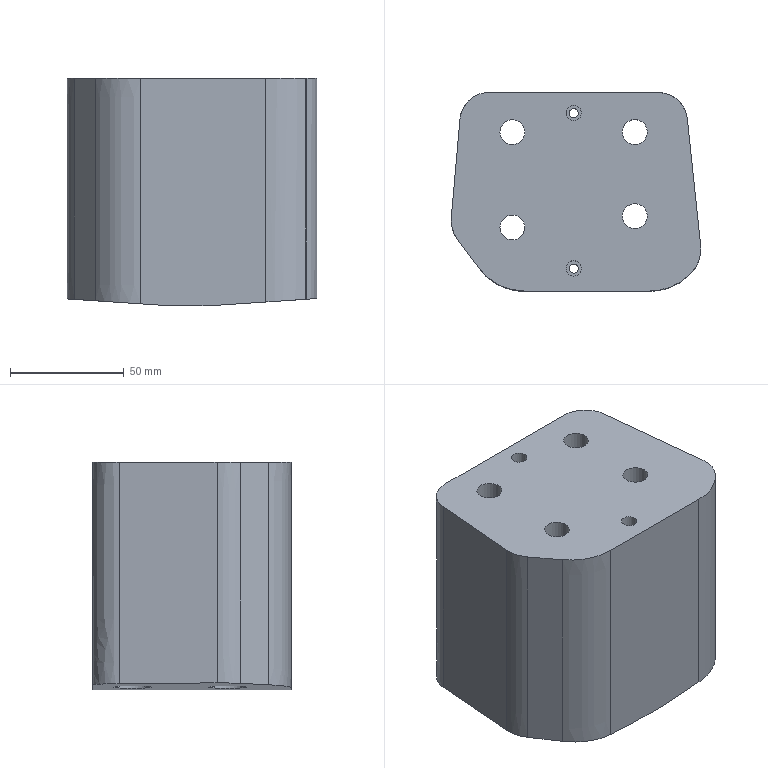Part | STEP file | lll_id3614_x_t | 1 solid | 42 faces | box 109.865 x 87.36 x 100 mm | volume 784858 mm3 | cylinder 18 | plane 18 | other 4 | cone 2 | commonest cylinder face diameters 11 x6 17 x4 4.1 x2 6.8 x2 8.506 x2 30 x1
STEP:
#1=CARTESIAN_POINT('',(3585.326,-140.05,29.5));
#2=VERTEX_POINT('',#1);
#3=CARTESIAN_POINT('',(3587.376,-140.05,29.5));
#4=DIRECTION('',(0.,0.,1.));
#5=DIRECTION('',(-1.,0.,0.));
#6=AXIS2_PLACEMENT_3D('',#3,#4,#5);
#7=CIRCLE('',#6,2.05);
#8=EDGE_CURVE('',#2,#2,#7,.T.);
#9=ORIENTED_EDGE('',*,*,#8,.T.);
#10=EDGE_LOOP('',(#9));
#11=FACE_BOUND('',#10,.T.);
#12=CARTESIAN_POINT('',(3587.376,-142.1,-7.5));
#13=VERTEX_POINT('',#12);
#14=CARTESIAN_POINT('',(3587.376,-140.05,-7.5));
#15=DIRECTION('',(0.,-0.000000008,-1.));
#16=DIRECTION('',(0.,-1.,0.000000008));
#17=AXIS2_PLACEMENT_3D('',#14,#15,#16);
#18=CIRCLE('',#17,2.05);
#19=EDGE_CURVE('',#13,#13,#18,.T.);
#20=ORIENTED_EDGE('',*,*,#19,.T.);
#21=EDGE_LOOP('',(#20));
#22=FACE_BOUND('',#21,.T.);
#23=CARTESIAN_POINT('',(3587.376,-140.05,42.5));
#24=DIRECTION('',(0.,0.,-1.));
#25=DIRECTION('',(0.,1.,0.));
#26=AXIS2_PLACEMENT_3D('',#23,#24,#25);
#27=CYLINDRICAL_SURFACE('',#26,2.05);
#28=ADVANCED_FACE('',(#11,#22),#27,.F.);
#29=CARTESIAN_POINT('',(3585.33,-71.615,29.5));
#30=VERTEX_POINT('',#29);
#31=CARTESIAN_POINT('',(3587.38,-71.615,29.5));
#32=DIRECTION('',(0.,0.,1.));
#33=DIRECTION('',(-1.,0.,0.));
#34=AXIS2_PLACEMENT_3D('',#31,#32,#33);
#35=CIRCLE('',#34,2.05);
#36=EDGE_CURVE('',#30,#30,#35,.T.);
#37=ORIENTED_EDGE('',*,*,#36,.T.);
#38=EDGE_LOOP('',(#37));
#39=FACE_BOUND('',#38,.T.);
#40=CARTESIAN_POINT('',(3587.38,-73.665,-7.5));
#41=VERTEX_POINT('',#40);
#42=CARTESIAN_POINT('',(3587.38,-71.615,-7.5));
#43=DIRECTION('',(0.,-0.000000008,-1.));
#44=DIRECTION('',(0.,-1.,0.000000008));
#45=AXIS2_PLACEMENT_3D('',#42,#43,#44);
#46=CIRCLE('',#45,2.05);
#47=EDGE_CURVE('',#41,#41,#46,.T.);
#48=ORIENTED_EDGE('',*,*,#47,.T.);
#49=EDGE_LOOP('',(#48));
#50=FACE_BOUND('',#49,.T.);
#51=CARTESIAN_POINT('',(3587.38,-71.615,42.5));
#52=DIRECTION('',(0.,0.,-1.));
#53=DIRECTION('',(-0.0006834,-1.,0.));
#54=AXIS2_PLACEMENT_3D('',#51,#52,#53);
#55=CYLINDRICAL_SURFACE('',#54,2.05);
#56=ADVANCED_FACE('',(#39,#50),#55,.F.);
#57=ORIENTED_EDGE('',*,*,#19,.F.);
#58=EDGE_LOOP('',(#57));
#59=FACE_BOUND('',#58,.T.);
#60=ORIENTED_EDGE('',*,*,#47,.F.);
#61=EDGE_LOOP('',(#60));
#62=FACE_BOUND('',#61,.T.);
#63=CARTESIAN_POINT('',(3587.38,-92.115,-7.5));
#64=VERTEX_POINT('',#63);
#65=CARTESIAN_POINT('',(3587.38,-86.615,-7.5));
#66=DIRECTION('',(0.,-0.000000008,-1.));
#67=DIRECTION('',(0.,-1.,0.000000008));
#68=AXIS2_PLACEMENT_3D('',#65,#66,#67);
#69=CIRCLE('',#68,5.5);
#70=EDGE_CURVE('',#64,#64,#69,.T.);
#71=ORIENTED_EDGE('',*,*,#70,.F.);
#72=EDGE_LOOP('',(#71));
#73=FACE_BOUND('',#72,.T.);
#74=CARTESIAN_POINT('',(3587.38,-130.115,-7.5));
#75=VERTEX_POINT('',#74);
#76=CARTESIAN_POINT('',(3587.38,-124.615,-7.5));
#77=DIRECTION('',(0.,-0.000000008,-1.));
#78=DIRECTION('',(0.,-1.,0.000000008));
#79=AXIS2_PLACEMENT_3D('',#76,#77,#78);
#80=CIRCLE('',#79,5.5);
#81=EDGE_CURVE('',#75,#75,#80,.T.);
#82=ORIENTED_EDGE('',*,*,#81,.F.);
#83=EDGE_LOOP('',(#82));
#84=FACE_BOUND('',#83,.T.);
#85=CARTESIAN_POINT('',(3597.232,-62.657,-7.5));
#86=VERTEX_POINT('',#85);
#87=CARTESIAN_POINT('',(3597.232,-150.017,-7.5));
#88=VERTEX_POINT('',#87);
#89=CARTESIAN_POINT('',(3597.232,-151.585,-7.5));
#90=DIRECTION('',(0.,-1.,0.));
#91=VECTOR('',#90,1.);
#92=LINE('',#89,#91);
#93=EDGE_CURVE('',#86,#88,#92,.T.);
#94=ORIENTED_EDGE('',*,*,#93,.T.);
#95=CARTESIAN_POINT('',(3577.232,-150.017,-7.5));
#96=VERTEX_POINT('',#95);
#97=CARTESIAN_POINT('',(3581.149,-150.017,-7.5));
#98=DIRECTION('',(-1.,0.,0.));
#99=VECTOR('',#98,1.);
#100=LINE('',#97,#99);
#101=EDGE_CURVE('',#88,#96,#100,.T.);
#102=ORIENTED_EDGE('',*,*,#101,.T.);
#103=CARTESIAN_POINT('',(3577.232,-62.657,-7.5));
#104=VERTEX_POINT('',#103);
#105=CARTESIAN_POINT('',(3577.232,-151.585,-7.5));
#106=DIRECTION('',(0.,-1.,0.));
#107=VECTOR('',#106,1.);
#108=LINE('',#105,#107);
#109=EDGE_CURVE('',#104,#96,#108,.T.);
#110=ORIENTED_EDGE('',*,*,#109,.F.);
#111=CARTESIAN_POINT('',(3587.337,-62.657,-7.5));
#112=DIRECTION('',(1.,0.,0.));
#113=VECTOR('',#112,1.);
#114=LINE('',#111,#113);
#115=EDGE_CURVE('',#104,#86,#114,.T.);
#116=ORIENTED_EDGE('',*,*,#115,.T.);
#117=EDGE_LOOP('',(#94,#102,#110,#116));
#118=FACE_BOUND('',#117,.T.);
#119=CARTESIAN_POINT('',(3633.202,65.944,-7.5));
#120=DIRECTION('',(0.,-0.000000008,1.));
#121=DIRECTION('',(0.,1.,0.000000008));
#122=AXIS2_PLACEMENT_3D('',#119,#120,#121);
#123=PLANE('',#122);
#124=ADVANCED_FACE('',(#59,#62,#73,#84,#118),#123,.F.);
#125=CARTESIAN_POINT('',(3638.938,-142.263,92.5));
#126=VERTEX_POINT('',#125);
#127=CARTESIAN_POINT('',(3638.507,-142.694,92.5));
#128=VERTEX_POINT('',#127);
#129=CARTESIAN_POINT('',(3802.568,21.366,92.5));
#130=DIRECTION('',(-0.7071,-0.7071,0.));
#131=VECTOR('',#130,1.);
#132=LINE('',#129,#131);
#133=EDGE_CURVE('',#126,#128,#132,.T.);
#134=ORIENTED_EDGE('',*,*,#133,.T.);
#135=CARTESIAN_POINT('',(3638.507,-142.694,-4.721));
#136=VERTEX_POINT('',#135);
#137=CARTESIAN_POINT('',(3638.507,-142.694,0.00002209));
#138=DIRECTION('',(0.000000008,0.,-1.));
#139=VECTOR('',#138,1.);
#140=LINE('',#137,#139);
#141=EDGE_CURVE('',#128,#136,#140,.T.);
#142=ORIENTED_EDGE('',*,*,#141,.T.);
#143=CARTESIAN_POINT('',(3638.938,-142.263,-4.692));
#144=VERTEX_POINT('',#143);
#145=CARTESIAN_POINT('',(3658.115,-123.087,-3.401));
#146=DIRECTION('',(0.7063,0.7063,0.04756));
#147=VECTOR('',#146,1.);
#148=LINE('',#145,#147);
#149=EDGE_CURVE('',#136,#144,#148,.T.);
#150=ORIENTED_EDGE('',*,*,#149,.T.);
#151=CARTESIAN_POINT('',(3638.938,-142.263,0.00002209));
#152=DIRECTION('',(-0.000000008,0.,1.));
#153=VECTOR('',#152,1.);
#154=LINE('',#151,#153);
#155=EDGE_CURVE('',#144,#126,#154,.T.);
#156=ORIENTED_EDGE('',*,*,#155,.T.);
#157=EDGE_LOOP('',(#134,#142,#150,#156));
#158=FACE_OUTER_BOUND('',#157,.T.);
#159=CARTESIAN_POINT('',(3638.507,-142.694,0.00002209));
#160=DIRECTION('',(-0.7071,0.7071,-0.000000005));
#161=DIRECTION('',(0.7071,0.7071,-0.000000005));
#162=AXIS2_PLACEMENT_3D('',#159,#160,#161);
#163=PLANE('',#162);
#164=ADVANCED_FACE('',(#158),#163,.F.);
#165=CARTESIAN_POINT('',(3637.367,-74.119,92.5));
#166=VERTEX_POINT('',#165);
#167=CARTESIAN_POINT('',(3643.25,-130.089,92.5));
#168=VERTEX_POINT('',#167);
#169=CARTESIAN_POINT('',(3639.152,-91.104,92.5));
#170=DIRECTION('',(0.1045,-0.9945,0.));
#171=VECTOR('',#170,1.);
#172=LINE('',#169,#171);
#173=EDGE_CURVE('',#166,#168,#172,.T.);
#174=ORIENTED_EDGE('',*,*,#173,.T.);
#175=CARTESIAN_POINT('',(3643.25,-130.089,-4.401));
#176=VERTEX_POINT('',#175);
#177=CARTESIAN_POINT('',(3643.25,-130.089,0.00001834));
#178=DIRECTION('',(0.000000008,0.,-1.));
#179=VECTOR('',#178,1.);
#180=LINE('',#177,#179);
#181=EDGE_CURVE('',#168,#176,#180,.T.);
#182=ORIENTED_EDGE('',*,*,#181,.T.);
#183=CARTESIAN_POINT('',(3637.367,-74.119,-4.798));
#184=VERTEX_POINT('',#183);
#185=CARTESIAN_POINT('',(3639.156,-91.136,-4.677));
#186=DIRECTION('',(-0.1045,0.9945,-0.007038));
#187=VECTOR('',#186,1.);
#188=LINE('',#185,#187);
#189=EDGE_CURVE('',#176,#184,#188,.T.);
#190=ORIENTED_EDGE('',*,*,#189,.T.);
#191=CARTESIAN_POINT('',(3637.367,-74.119,0.00001829));
#192=DIRECTION('',(-0.000000008,0.,1.));
#193=VECTOR('',#192,1.);
#194=LINE('',#191,#193);
#195=EDGE_CURVE('',#184,#166,#194,.T.);
#196=ORIENTED_EDGE('',*,*,#195,.T.);
#197=EDGE_LOOP('',(#174,#182,#190,#196));
#198=FACE_OUTER_BOUND('',#197,.T.);
#199=CARTESIAN_POINT('',(3639.152,-91.104,0.00001831));
#200=DIRECTION('',(-0.9945,-0.1045,-0.000000008));
#201=DIRECTION('',(0.1045,-0.9945,0.000000001));
#202=AXIS2_PLACEMENT_3D('',#199,#200,#201);
#203=PLANE('',#202);
#204=ADVANCED_FACE('',(#198),#203,.F.);
#205=ORIENTED_EDGE('',*,*,#195,.F.);
#206=CARTESIAN_POINT('',(3624.637,-62.657,-5.655));
#207=VERTEX_POINT('',#206);
#208=CARTESIAN_POINT('',(3637.367,-74.119,-4.798));
#209=CARTESIAN_POINT('',(3637.037,-70.978,-4.82));
#210=CARTESIAN_POINT('',(3635.528,-68.038,-4.921));
#211=CARTESIAN_POINT('',(3630.875,-63.85,-5.235));
#212=CARTESIAN_POINT('',(3627.791,-62.657,-5.442));
#213=CARTESIAN_POINT('',(3624.637,-62.657,-5.655));
#214=B_SPLINE_CURVE_WITH_KNOTS('',3,(#208,#209,#210,#211,#212,#213),.UNSPECIFIED.,.F.,.F.,(4,2,4),(0.,0.5,1.),.UNSPECIFIED.);
#215=EDGE_CURVE('',#184,#207,#214,.T.);
#216=ORIENTED_EDGE('',*,*,#215,.T.);
#217=CARTESIAN_POINT('',(3624.637,-62.657,92.5));
#218=VERTEX_POINT('',#217);
#219=CARTESIAN_POINT('',(3624.637,-62.657,0.0000182));
#220=DIRECTION('',(-0.000000008,0.,1.));
#221=VECTOR('',#220,1.);
#222=LINE('',#219,#221);
#223=EDGE_CURVE('',#207,#218,#222,.T.);
#224=ORIENTED_EDGE('',*,*,#223,.T.);
#225=CARTESIAN_POINT('',(3624.637,-62.657,92.5));
#226=CARTESIAN_POINT('',(3627.791,-62.657,92.5));
#227=CARTESIAN_POINT('',(3630.87,-63.847,92.5));
#228=CARTESIAN_POINT('',(3635.525,-68.034,92.5));
#229=CARTESIAN_POINT('',(3637.037,-70.978,92.5));
#230=CARTESIAN_POINT('',(3637.367,-74.119,92.5));
#231=B_SPLINE_CURVE_WITH_KNOTS('',3,(#225,#226,#227,#228,#229,#230),.UNSPECIFIED.,.F.,.F.,(4,2,4),(0.,0.5,1.),.UNSPECIFIED.);
#232=EDGE_CURVE('',#218,#166,#231,.T.);
#233=ORIENTED_EDGE('',*,*,#232,.T.);
#234=EDGE_LOOP('',(#205,#216,#224,#233));
#235=FACE_OUTER_BOUND('',#234,.T.);
#236=CARTESIAN_POINT('',(3624.637,-62.657,0.0000182));
#237=CARTESIAN_POINT('',(3625.028,-62.657,0.0000182));
#238=CARTESIAN_POINT('',(3625.81,-62.691,0.00001821));
#239=CARTESIAN_POINT('',(3627.361,-62.904,0.00001822));
#240=CARTESIAN_POINT('',(3629.249,-63.441,0.00001823));
#241=CARTESIAN_POINT('',(3631.364,-64.478,0.00001825));
#242=CARTESIAN_POINT('',(3633.249,-65.892,0.00001826));
#243=CARTESIAN_POINT('',(3634.852,-67.618,0.00001828));
#244=CARTESIAN_POINT('',(3636.105,-69.613,0.00001828));
#245=CARTESIAN_POINT('',(3636.836,-71.435,0.00001829));
#246=CARTESIAN_POINT('',(3637.21,-72.956,0.00001829));
#247=CARTESIAN_POINT('',(3637.326,-73.73,0.00001829));
#248=CARTESIAN_POINT('',(3637.367,-74.119,0.00001829));
#249=B_SPLINE_CURVE_WITH_KNOTS('',3,(#236,#237,#238,#239,#240,#241,#242,#243,#244,#245,#246,#247,#248),.UNSPECIFIED.,.F.,.F.,(4,1,1,1,1,1,1,1,1,1,4),(0.,0.0625,0.125,0.25,0.375,0.5,0.625,0.75,0.875,0.9375,1.),.UNSPECIFIED.);
#250=DIRECTION('',(-0.000000008,0.,1.));
#251=VECTOR('',#250,1.);
#252=SURFACE_OF_LINEAR_EXTRUSION('',#249,#251);
#253=ADVANCED_FACE('',(#235),#252,.F.);
#254=CARTESIAN_POINT('',(3550.037,-62.657,-5.669));
#255=VERTEX_POINT('',#254);
#256=CARTESIAN_POINT('',(3586.789,-62.657,-8.143));
#257=DIRECTION('',(0.9977,0.,-0.06718));
#258=VECTOR('',#257,1.);
#259=LINE('',#256,#258);
#260=EDGE_CURVE('',#255,#104,#259,.T.);
#261=ORIENTED_EDGE('',*,*,#260,.F.);
#262=CARTESIAN_POINT('',(3550.037,-62.657,92.5));
#263=VERTEX_POINT('',#262);
#264=CARTESIAN_POINT('',(3550.037,-62.657,0.00001763));
#265=DIRECTION('',(-0.000000008,0.,1.));
#266=VECTOR('',#265,1.);
#267=LINE('',#264,#266);
#268=EDGE_CURVE('',#255,#263,#267,.T.);
#269=ORIENTED_EDGE('',*,*,#268,.T.);
#270=CARTESIAN_POINT('',(3587.337,-62.657,92.5));
#271=DIRECTION('',(1.,0.,0.));
#272=VECTOR('',#271,1.);
#273=LINE('',#270,#272);
#274=EDGE_CURVE('',#263,#218,#273,.T.);
#275=ORIENTED_EDGE('',*,*,#274,.T.);
#276=ORIENTED_EDGE('',*,*,#223,.F.);
#277=CARTESIAN_POINT('',(3587.884,-62.657,-8.129));
#278=DIRECTION('',(-0.9977,0.,-0.06718));
#279=VECTOR('',#278,1.);
#280=LINE('',#277,#279);
#281=EDGE_CURVE('',#207,#86,#280,.T.);
#282=ORIENTED_EDGE('',*,*,#281,.T.);
#283=ORIENTED_EDGE('',*,*,#115,.F.);
#284=EDGE_LOOP('',(#261,#269,#275,#276,#282,#283));
#285=FACE_OUTER_BOUND('',#284,.T.);
#286=CARTESIAN_POINT('',(3587.337,-62.657,0.00001792));
#287=DIRECTION('',(0.,-1.,0.));
#288=DIRECTION('',(1.,0.,0.000000008));
#289=AXIS2_PLACEMENT_3D('',#286,#287,#288);
#290=PLANE('',#289);
#291=ADVANCED_FACE('',(#285),#290,.F.);
#292=CARTESIAN_POINT('',(3614.279,-71.531,62.5));
#293=VERTEX_POINT('',#292);
#294=CARTESIAN_POINT('',(3614.279,-80.031,62.5));
#295=DIRECTION('',(0.,0.,1.));
#296=DIRECTION('',(0.,1.,0.));
#297=AXIS2_PLACEMENT_3D('',#294,#295,#296);
#298=CIRCLE('',#297,8.5);
#299=EDGE_CURVE('',#293,#293,#298,.T.);
#300=ORIENTED_EDGE('',*,*,#299,.T.);
#301=EDGE_LOOP('',(#300));
#302=FACE_BOUND('',#301,.T.);
#303=CARTESIAN_POINT('',(3622.779,-80.031,-5.78));
#304=VERTEX_POINT('',#303);
#305=CARTESIAN_POINT('',(3614.279,-80.031,-6.352));
#306=DIRECTION('',(-0.06718,0.,0.9977));
#307=DIRECTION('',(0.9977,0.,0.06718));
#308=AXIS2_PLACEMENT_3D('',#305,#306,#307);
#309=ELLIPSE('',#308,8.519,8.5);
#310=EDGE_CURVE('',#304,#304,#309,.T.);
#311=ORIENTED_EDGE('',*,*,#310,.F.);
#312=EDGE_LOOP('',(#311));
#313=FACE_BOUND('',#312,.T.);
#314=CARTESIAN_POINT('',(3614.279,-80.031,12.5));
#315=DIRECTION('',(0.,0.,1.));
#316=DIRECTION('',(0.,-1.,0.));
#317=AXIS2_PLACEMENT_3D('',#314,#315,#316);
#318=CYLINDRICAL_SURFACE('',#317,8.5);
#319=ADVANCED_FACE('',(#302,#313),#318,.F.);
#320=CARTESIAN_POINT('',(3614.279,-108.531,62.5));
#321=VERTEX_POINT('',#320);
#322=CARTESIAN_POINT('',(3614.279,-117.031,62.5));
#323=DIRECTION('',(0.,0.,1.));
#324=DIRECTION('',(0.,1.,0.));
#325=AXIS2_PLACEMENT_3D('',#322,#323,#324);
#326=CIRCLE('',#325,8.5);
#327=EDGE_CURVE('',#321,#321,#326,.T.);
#328=ORIENTED_EDGE('',*,*,#327,.T.);
#329=EDGE_LOOP('',(#328));
#330=FACE_BOUND('',#329,.T.);
#331=CARTESIAN_POINT('',(3622.779,-117.031,-5.78));
#332=VERTEX_POINT('',#331);
#333=CARTESIAN_POINT('',(3614.279,-117.031,-6.352));
#334=DIRECTION('',(-0.06718,0.,0.9977));
#335=DIRECTION('',(0.9977,0.,0.06718));
#336=AXIS2_PLACEMENT_3D('',#333,#334,#335);
#337=ELLIPSE('',#336,8.519,8.5);
#338=EDGE_CURVE('',#332,#332,#337,.T.);
#339=ORIENTED_EDGE('',*,*,#338,.F.);
#340=EDGE_LOOP('',(#339));
#341=FACE_BOUND('',#340,.T.);
#342=CARTESIAN_POINT('',(3614.279,-117.031,12.5));
#343=DIRECTION('',(0.,0.,1.));
#344=DIRECTION('',(0.,-1.,0.));
#345=AXIS2_PLACEMENT_3D('',#342,#343,#344);
#346=CYLINDRICAL_SURFACE('',#345,8.5);
#347=ADVANCED_FACE('',(#330,#341),#346,.F.);
#348=CARTESIAN_POINT('',(3554.876,-80.05,92.5));
#349=VERTEX_POINT('',#348);
#350=CARTESIAN_POINT('',(3560.376,-80.05,92.5));
#351=DIRECTION('',(0.,0.,1.));
#352=DIRECTION('',(-1.,0.,0.));
#353=AXIS2_PLACEMENT_3D('',#350,#351,#352);
#354=CIRCLE('',#353,5.5);
#355=EDGE_CURVE('',#349,#349,#354,.T.);
#356=ORIENTED_EDGE('',*,*,#355,.F.);
#357=EDGE_LOOP('',(#356));
#358=FACE_BOUND('',#357,.T.);
#359=CARTESIAN_POINT('',(3620.83,-150.017,92.5));
#360=VERTEX_POINT('',#359);
#361=CARTESIAN_POINT('',(3565.78,-150.017,92.5));
#362=VERTEX_POINT('',#361);
#363=CARTESIAN_POINT('',(3581.149,-150.017,92.5));
#364=DIRECTION('',(-1.,0.,0.));
#365=VECTOR('',#364,1.);
#366=LINE('',#363,#365);
#367=EDGE_CURVE('',#360,#362,#366,.T.);
#368=ORIENTED_EDGE('',*,*,#367,.F.);
#369=CARTESIAN_POINT('',(3620.83,-125.017,92.5));
#370=DIRECTION('',(0.,0.,1.));
#371=DIRECTION('',(1.,0.,0.));
#372=AXIS2_PLACEMENT_3D('',#369,#370,#371);
#373=CIRCLE('',#372,25.);
#374=EDGE_CURVE('',#360,#128,#373,.T.);
#375=ORIENTED_EDGE('',*,*,#374,.T.);
#376=ORIENTED_EDGE('',*,*,#133,.F.);
#377=CARTESIAN_POINT('',(3628.332,-131.657,92.5));
#378=DIRECTION('',(0.,0.,1.));
#379=DIRECTION('',(1.,0.,0.));
#380=AXIS2_PLACEMENT_3D('',#377,#378,#379);
#381=CIRCLE('',#380,15.);
#382=EDGE_CURVE('',#126,#168,#381,.T.);
#383=ORIENTED_EDGE('',*,*,#382,.T.);
#384=ORIENTED_EDGE('',*,*,#173,.F.);
#385=ORIENTED_EDGE('',*,*,#232,.F.);
#386=ORIENTED_EDGE('',*,*,#274,.F.);
#387=CARTESIAN_POINT('',(3537.286,-74.341,92.5));
#388=VERTEX_POINT('',#387);
#389=CARTESIAN_POINT('',(3537.286,-74.341,92.5));
#390=CARTESIAN_POINT('',(3537.564,-71.162,92.5));
#391=CARTESIAN_POINT('',(3539.052,-68.163,92.5));
#392=CARTESIAN_POINT('',(3543.717,-63.885,92.5));
#393=CARTESIAN_POINT('',(3546.842,-62.657,92.5));
#394=CARTESIAN_POINT('',(3550.037,-62.657,92.5));
#395=B_SPLINE_CURVE_WITH_KNOTS('',3,(#389,#390,#391,#392,#393,#394),.UNSPECIFIED.,.F.,.F.,(4,2,4),(0.,0.5,1.),.UNSPECIFIED.);
#396=EDGE_CURVE('',#388,#263,#395,.T.);
#397=ORIENTED_EDGE('',*,*,#396,.F.);
#398=CARTESIAN_POINT('',(3533.523,-117.349,92.5));
#399=VERTEX_POINT('',#398);
#400=CARTESIAN_POINT('',(3535.404,-95.845,92.5));
#401=DIRECTION('',(0.08716,0.9962,0.));
#402=VECTOR('',#401,1.);
#403=LINE('',#400,#402);
#404=EDGE_CURVE('',#399,#388,#403,.T.);
#405=ORIENTED_EDGE('',*,*,#404,.F.);
#406=CARTESIAN_POINT('',(3536.486,-127.684,92.5));
#407=VERTEX_POINT('',#406);
#408=CARTESIAN_POINT('',(3536.486,-127.684,92.5));
#409=CARTESIAN_POINT('',(3534.267,-124.738,92.5));
#410=CARTESIAN_POINT('',(3533.202,-121.023,92.5));
#411=CARTESIAN_POINT('',(3533.523,-117.349,92.5));
#412=B_SPLINE_CURVE_WITH_KNOTS('',3,(#408,#409,#410,#411),.UNSPECIFIED.,.F.,.F.,(4,4),(0.,1.),.UNSPECIFIED.);
#413=EDGE_CURVE('',#407,#399,#412,.T.);
#414=ORIENTED_EDGE('',*,*,#413,.F.);
#415=CARTESIAN_POINT('',(3545.814,-140.062,92.5));
#416=VERTEX_POINT('',#415);
#417=CARTESIAN_POINT('',(3541.15,-133.873,92.5));
#418=DIRECTION('',(-0.6018,0.7986,0.));
#419=VECTOR('',#418,1.);
#420=LINE('',#417,#419);
#421=EDGE_CURVE('',#416,#407,#420,.T.);
#422=ORIENTED_EDGE('',*,*,#421,.F.);
#423=CARTESIAN_POINT('',(3565.78,-150.017,92.5));
#424=CARTESIAN_POINT('',(3561.891,-150.017,92.5));
#425=CARTESIAN_POINT('',(3558.048,-149.099,92.5));
#426=CARTESIAN_POINT('',(3552.892,-146.525,92.5));
#427=CARTESIAN_POINT('',(3551.245,-145.458,92.5));
#428=CARTESIAN_POINT('',(3548.301,-143.006,92.5));
#429=CARTESIAN_POINT('',(3546.983,-141.614,92.5));
#430=CARTESIAN_POINT('',(3545.814,-140.062,92.5));
#431=B_SPLINE_CURVE_WITH_KNOTS('',3,(#423,#424,#425,#426,#427,#428,#429,#430),.UNSPECIFIED.,.F.,.F.,(4,2,2,4),(0.,0.5,0.75,1.),.UNSPECIFIED.);
#432=EDGE_CURVE('',#362,#416,#431,.T.);
#433=ORIENTED_EDGE('',*,*,#432,.F.);
#434=EDGE_LOOP('',(#368,#375,#376,#383,#384,#385,#386,#397,#405,#414,#422,#433));
#435=FACE_BOUND('',#434,.T.);
#436=CARTESIAN_POINT('',(3587.378,-75.015,92.5));
#437=VERTEX_POINT('',#436);
#438=CARTESIAN_POINT('',(3587.38,-71.615,92.5));
#439=DIRECTION('',(0.,0.,-1.));
#440=DIRECTION('',(-0.0006834,-1.,0.));
#441=AXIS2_PLACEMENT_3D('',#438,#439,#440);
#442=CIRCLE('',#441,3.4);
#443=EDGE_CURVE('',#437,#437,#442,.T.);
#444=ORIENTED_EDGE('',*,*,#443,.T.);
#445=EDGE_LOOP('',(#444));
#446=FACE_BOUND('',#445,.T.);
#447=CARTESIAN_POINT('',(3587.376,-136.65,92.5));
#448=VERTEX_POINT('',#447);
#449=CARTESIAN_POINT('',(3587.376,-140.05,92.5));
#450=DIRECTION('',(0.,0.,1.));
#451=DIRECTION('',(0.,1.,0.));
#452=AXIS2_PLACEMENT_3D('',#449,#450,#451);
#453=CIRCLE('',#452,3.4);
#454=EDGE_CURVE('',#448,#448,#453,.T.);
#455=ORIENTED_EDGE('',*,*,#454,.F.);
#456=EDGE_LOOP('',(#455));
#457=FACE_BOUND('',#456,.T.);
#458=CARTESIAN_POINT('',(3608.779,-80.031,92.5));
#459=VERTEX_POINT('',#458);
#460=CARTESIAN_POINT('',(3614.279,-80.031,92.5));
#461=DIRECTION('',(0.,0.,-1.));
#462=DIRECTION('',(-1.,0.,0.));
#463=AXIS2_PLACEMENT_3D('',#460,#461,#462);
#464=CIRCLE('',#463,5.5);
#465=EDGE_CURVE('',#459,#459,#464,.T.);
#466=ORIENTED_EDGE('',*,*,#465,.T.);
#467=EDGE_LOOP('',(#466));
#468=FACE_BOUND('',#467,.T.);
#469=CARTESIAN_POINT('',(3608.779,-117.031,92.5));
#470=VERTEX_POINT('',#469);
#471=CARTESIAN_POINT('',(3614.279,-117.031,92.5));
#472=DIRECTION('',(0.,0.,-1.));
#473=DIRECTION('',(-1.,0.,0.));
#474=AXIS2_PLACEMENT_3D('',#471,#472,#473);
#475=CIRCLE('',#474,5.5);
#476=EDGE_CURVE('',#470,#470,#475,.T.);
#477=ORIENTED_EDGE('',*,*,#476,.T.);
#478=EDGE_LOOP('',(#477));
#479=FACE_BOUND('',#478,.T.);
#480=CARTESIAN_POINT('',(3554.876,-122.05,92.5));
#481=VERTEX_POINT('',#480);
#482=CARTESIAN_POINT('',(3560.376,-122.05,92.5));
#483=DIRECTION('',(0.,0.,-1.));
#484=DIRECTION('',(-1.,0.,0.));
#485=AXIS2_PLACEMENT_3D('',#482,#483,#484);
#486=CIRCLE('',#485,5.5);
#487=EDGE_CURVE('',#481,#481,#486,.T.);
#488=ORIENTED_EDGE('',*,*,#487,.T.);
#489=EDGE_LOOP('',(#488));
#490=FACE_BOUND('',#489,.T.);
#491=CARTESIAN_POINT('',(3587.234,236.7,92.5));
#492=DIRECTION('',(0.,0.,1.));
#493=DIRECTION('',(0.,-1.,0.));
#494=AXIS2_PLACEMENT_3D('',#491,#492,#493);
#495=PLANE('',#494);
#496=ADVANCED_FACE('',(#358,#435,#446,#457,#468,#479,#490),#495,.T.);
#497=CARTESIAN_POINT('',(3620.83,-150.017,-5.911));
#498=VERTEX_POINT('',#497);
#499=CARTESIAN_POINT('',(3581.724,-150.017,-8.544));
#500=DIRECTION('',(-0.9977,0.,-0.06718));
#501=VECTOR('',#500,1.);
#502=LINE('',#499,#501);
#503=EDGE_CURVE('',#498,#88,#502,.T.);
#504=ORIENTED_EDGE('',*,*,#503,.F.);
#505=CARTESIAN_POINT('',(3620.83,-150.017,0.00001817));
#506=DIRECTION('',(-0.000000008,0.,1.));
#507=VECTOR('',#506,1.);
#508=LINE('',#505,#507);
#509=EDGE_CURVE('',#498,#360,#508,.T.);
#510=ORIENTED_EDGE('',*,*,#509,.T.);
#511=ORIENTED_EDGE('',*,*,#367,.T.);
#512=CARTESIAN_POINT('',(3565.78,-150.017,-6.729));
#513=VERTEX_POINT('',#512);
#514=CARTESIAN_POINT('',(3565.78,-150.017,0.00001775));
#515=DIRECTION('',(-0.000000008,0.,1.));
#516=VECTOR('',#515,1.);
#517=LINE('',#514,#516);
#518=EDGE_CURVE('',#513,#362,#517,.T.);
#519=ORIENTED_EDGE('',*,*,#518,.F.);
#520=CARTESIAN_POINT('',(3580.628,-150.017,-7.729));
#521=DIRECTION('',(-0.9977,0.,0.06718));
#522=VECTOR('',#521,1.);
#523=LINE('',#520,#522);
#524=EDGE_CURVE('',#96,#513,#523,.T.);
#525=ORIENTED_EDGE('',*,*,#524,.F.);
#526=ORIENTED_EDGE('',*,*,#101,.F.);
#527=EDGE_LOOP('',(#504,#510,#511,#519,#525,#526));
#528=FACE_OUTER_BOUND('',#527,.T.);
#529=CARTESIAN_POINT('',(3581.149,-150.017,0.00001787));
#530=DIRECTION('',(0.,1.,0.));
#531=DIRECTION('',(-1.,0.,-0.000000008));
#532=AXIS2_PLACEMENT_3D('',#529,#530,#531);
#533=PLANE('',#532);
#534=ADVANCED_FACE('',(#528),#533,.F.);
#535=CARTESIAN_POINT('',(3537.286,-74.341,-4.81));
#536=VERTEX_POINT('',#535);
#537=CARTESIAN_POINT('',(3550.037,-62.657,-5.669));
#538=CARTESIAN_POINT('',(3546.849,-62.657,-5.454));
#539=CARTESIAN_POINT('',(3543.735,-63.874,-5.245));
#540=CARTESIAN_POINT('',(3539.063,-68.147,-4.93));
#541=CARTESIAN_POINT('',(3537.565,-71.154,-4.829));
#542=CARTESIAN_POINT('',(3537.286,-74.341,-4.81));
#543=B_SPLINE_CURVE_WITH_KNOTS('',3,(#537,#538,#539,#540,#541,#542),.UNSPECIFIED.,.F.,.F.,(4,2,4),(0.,0.5,1.),.UNSPECIFIED.);
#544=EDGE_CURVE('',#255,#536,#543,.T.);
#545=ORIENTED_EDGE('',*,*,#544,.T.);
#546=CARTESIAN_POINT('',(3537.286,-74.341,0.00001754));
#547=DIRECTION('',(-0.000000008,0.,1.));
#548=VECTOR('',#547,1.);
#549=LINE('',#546,#548);
#550=EDGE_CURVE('',#536,#388,#549,.T.);
#551=ORIENTED_EDGE('',*,*,#550,.T.);
#552=ORIENTED_EDGE('',*,*,#396,.T.);
#553=ORIENTED_EDGE('',*,*,#268,.F.);
#554=EDGE_LOOP('',(#545,#551,#552,#553));
#555=FACE_OUTER_BOUND('',#554,.T.);
#556=CARTESIAN_POINT('',(3537.286,-74.341,0.00001754));
#557=CARTESIAN_POINT('',(3537.32,-73.947,0.00001754));
#558=CARTESIAN_POINT('',(3537.425,-73.162,0.00001754));
#559=CARTESIAN_POINT('',(3537.778,-71.617,0.00001754));
#560=CARTESIAN_POINT('',(3538.492,-69.763,0.00001755));
#561=CARTESIAN_POINT('',(3539.736,-67.729,0.00001755));
#562=CARTESIAN_POINT('',(3541.341,-65.967,0.00001757));
#563=CARTESIAN_POINT('',(3543.237,-64.521,0.00001758));
#564=CARTESIAN_POINT('',(3545.372,-63.46,0.0000176));
#565=CARTESIAN_POINT('',(3547.281,-62.91,0.00001761));
#566=CARTESIAN_POINT('',(3548.85,-62.692,0.00001762));
#567=CARTESIAN_POINT('',(3549.641,-62.657,0.00001763));
#568=CARTESIAN_POINT('',(3550.037,-62.657,0.00001763));
#569=B_SPLINE_CURVE_WITH_KNOTS('',3,(#556,#557,#558,#559,#560,#561,#562,#563,#564,#565,#566,#567,#568),.UNSPECIFIED.,.F.,.F.,(4,1,1,1,1,1,1,1,1,1,4),(0.,0.0625,0.125,0.25,0.375,0.5,0.625,0.75,0.875,0.9375,1.),.UNSPECIFIED.);
#570=DIRECTION('',(-0.000000008,0.,1.));
#571=VECTOR('',#570,1.);
#572=SURFACE_OF_LINEAR_EXTRUSION('',#569,#571);
#573=ADVANCED_FACE('',(#555),#572,.F.);
#574=CARTESIAN_POINT('',(3533.523,-117.349,-4.557));
#575=VERTEX_POINT('',#574);
#576=CARTESIAN_POINT('',(3535.402,-95.872,-4.683));
#577=DIRECTION('',(-0.08715,-0.9962,0.005868));
#578=VECTOR('',#577,1.);
#579=LINE('',#576,#578);
#580=EDGE_CURVE('',#536,#575,#579,.T.);
#581=ORIENTED_EDGE('',*,*,#580,.T.);
#582=CARTESIAN_POINT('',(3533.523,-117.349,0.00001751));
#583=DIRECTION('',(-0.000000008,0.,1.));
#584=VECTOR('',#583,1.);
#585=LINE('',#582,#584);
#586=EDGE_CURVE('',#575,#399,#585,.T.);
#587=ORIENTED_EDGE('',*,*,#586,.T.);
#588=ORIENTED_EDGE('',*,*,#404,.T.);
#589=ORIENTED_EDGE('',*,*,#550,.F.);
#590=EDGE_LOOP('',(#581,#587,#588,#589));
#591=FACE_OUTER_BOUND('',#590,.T.);
#592=CARTESIAN_POINT('',(3535.404,-95.845,0.00001752));
#593=DIRECTION('',(0.9962,-0.08716,0.000000008));
#594=DIRECTION('',(0.08716,0.9962,0.000000001));
#595=AXIS2_PLACEMENT_3D('',#592,#593,#594);
#596=PLANE('',#595);
#597=ADVANCED_FACE('',(#591),#596,.F.);
#598=CARTESIAN_POINT('',(3536.486,-127.684,-4.756));
#599=VERTEX_POINT('',#598);
#600=CARTESIAN_POINT('',(3533.523,-117.349,-4.557));
#601=CARTESIAN_POINT('',(3533.202,-121.024,-4.535));
#602=CARTESIAN_POINT('',(3534.268,-124.74,-4.607));
#603=CARTESIAN_POINT('',(3536.486,-127.684,-4.756));
#604=B_SPLINE_CURVE_WITH_KNOTS('',3,(#600,#601,#602,#603),.UNSPECIFIED.,.F.,.F.,(4,4),(0.,1.),.UNSPECIFIED.);
#605=EDGE_CURVE('',#575,#599,#604,.T.);
#606=ORIENTED_EDGE('',*,*,#605,.T.);
#607=CARTESIAN_POINT('',(3536.486,-127.684,0.00001753));
#608=DIRECTION('',(-0.000000008,0.,1.));
#609=VECTOR('',#608,1.);
#610=LINE('',#607,#609);
#611=EDGE_CURVE('',#599,#407,#610,.T.);
#612=ORIENTED_EDGE('',*,*,#611,.T.);
#613=ORIENTED_EDGE('',*,*,#413,.T.);
#614=ORIENTED_EDGE('',*,*,#586,.F.);
#615=EDGE_LOOP('',(#606,#612,#613,#614));
#616=FACE_OUTER_BOUND('',#615,.T.);
#617=CARTESIAN_POINT('',(3536.486,-127.684,0.00001753));
#618=CARTESIAN_POINT('',(3536.211,-127.318,0.00001753));
#619=CARTESIAN_POINT('',(3535.692,-126.561,0.00001752));
#620=CARTESIAN_POINT('',(3535.021,-125.36,0.00001752));
#621=CARTESIAN_POINT('',(3534.465,-124.101,0.00001751));
#622=CARTESIAN_POINT('',(3534.027,-122.797,0.00001751));
#623=CARTESIAN_POINT('',(3533.707,-121.458,0.00001751));
#624=CARTESIAN_POINT('',(3533.511,-120.096,0.00001751));
#625=CARTESIAN_POINT('',(3533.444,-118.722,0.00001751));
#626=CARTESIAN_POINT('',(3533.483,-117.806,0.00001751));
#627=CARTESIAN_POINT('',(3533.523,-117.349,0.00001751));
#628=B_SPLINE_CURVE_WITH_KNOTS('',3,(#617,#618,#619,#620,#621,#622,#623,#624,#625,#626,#627),.UNSPECIFIED.,.F.,.F.,(4,1,1,1,1,1,1,1,4),(0.,0.125,0.25,0.375,0.5,0.625,0.75,0.875,1.),.UNSPECIFIED.);
#629=DIRECTION('',(-0.000000008,0.,1.));
#630=VECTOR('',#629,1.);
#631=SURFACE_OF_LINEAR_EXTRUSION('',#628,#630);
#632=ADVANCED_FACE('',(#616),#631,.F.);
#633=CARTESIAN_POINT('',(3545.814,-140.062,-5.385));
#634=VERTEX_POINT('',#633);
#635=CARTESIAN_POINT('',(3541.027,-133.709,-5.062));
#636=DIRECTION('',(0.6013,-0.798,-0.04049));
#637=VECTOR('',#636,1.);
#638=LINE('',#635,#637);
#639=EDGE_CURVE('',#599,#634,#638,.T.);
#640=ORIENTED_EDGE('',*,*,#639,.T.);
#641=CARTESIAN_POINT('',(3545.814,-140.062,0.0000176));
#642=DIRECTION('',(-0.000000008,0.,1.));
#643=VECTOR('',#642,1.);
#644=LINE('',#641,#643);
#645=EDGE_CURVE('',#634,#416,#644,.T.);
#646=ORIENTED_EDGE('',*,*,#645,.T.);
#647=ORIENTED_EDGE('',*,*,#421,.T.);
#648=ORIENTED_EDGE('',*,*,#611,.F.);
#649=EDGE_LOOP('',(#640,#646,#647,#648));
#650=FACE_OUTER_BOUND('',#649,.T.);
#651=CARTESIAN_POINT('',(3541.15,-133.873,0.00001757));
#652=DIRECTION('',(0.7986,0.6018,0.000000006));
#653=DIRECTION('',(-0.6018,0.7986,-0.000000005));
#654=AXIS2_PLACEMENT_3D('',#651,#652,#653);
#655=PLANE('',#654);
#656=ADVANCED_FACE('',(#650),#655,.F.);
#657=CARTESIAN_POINT('',(3545.814,-140.062,-5.385));
#658=CARTESIAN_POINT('',(3548.156,-143.17,-5.542));
#659=CARTESIAN_POINT('',(3551.204,-145.688,-5.747));
#660=CARTESIAN_POINT('',(3556.362,-148.255,-6.095));
#661=CARTESIAN_POINT('',(3558.205,-148.928,-6.219));
#662=CARTESIAN_POINT('',(3561.934,-149.803,-6.47));
#663=CARTESIAN_POINT('',(3563.838,-150.017,-6.598));
#664=CARTESIAN_POINT('',(3565.78,-150.017,-6.729));
#665=B_SPLINE_CURVE_WITH_KNOTS('',3,(#657,#658,#659,#660,#661,#662,#663,#664),.UNSPECIFIED.,.F.,.F.,(4,2,2,4),(0.,0.5,0.75,1.),.UNSPECIFIED.);
#666=EDGE_CURVE('',#634,#513,#665,.T.);
#667=ORIENTED_EDGE('',*,*,#666,.T.);
#668=ORIENTED_EDGE('',*,*,#518,.T.);
#669=ORIENTED_EDGE('',*,*,#432,.T.);
#670=ORIENTED_EDGE('',*,*,#645,.F.);
#671=EDGE_LOOP('',(#667,#668,#669,#670));
#672=FACE_OUTER_BOUND('',#671,.T.);
#673=CARTESIAN_POINT('',(3565.78,-150.017,0.00001775));
#674=CARTESIAN_POINT('',(3565.298,-150.017,0.00001775));
#675=CARTESIAN_POINT('',(3564.334,-149.99,0.00001774));
#676=CARTESIAN_POINT('',(3562.413,-149.828,0.00001773));
#677=CARTESIAN_POINT('',(3560.034,-149.416,0.00001771));
#678=CARTESIAN_POINT('',(3557.723,-148.723,0.00001769));
#679=CARTESIAN_POINT('',(3555.931,-148.011,0.00001768));
#680=CARTESIAN_POINT('',(3554.619,-147.402,0.00001767));
#681=CARTESIAN_POINT('',(3553.343,-146.721,0.00001766));
#682=CARTESIAN_POINT('',(3551.696,-145.718,0.00001765));
#683=CARTESIAN_POINT('',(3549.751,-144.289,0.00001763));
#684=CARTESIAN_POINT('',(3547.991,-142.638,0.00001762));
#685=CARTESIAN_POINT('',(3546.705,-141.201,0.00001761));
#686=CARTESIAN_POINT('',(3546.104,-140.447,0.0000176));
#687=CARTESIAN_POINT('',(3545.814,-140.062,0.0000176));
#688=B_SPLINE_CURVE_WITH_KNOTS('',3,(#673,#674,#675,#676,#677,#678,#679,#680,#681,#682,#683,#684,#685,#686,#687),.UNSPECIFIED.,.F.,.F.,(4,1,1,1,1,1,1,1,1,1,1,1,4),(0.,0.0625,0.125,0.25,0.375,0.4375,0.5,0.5625,0.625,0.75,0.875,0.9375,1.),.UNSPECIFIED.);
#689=DIRECTION('',(-0.000000008,0.,1.));
#690=VECTOR('',#689,1.);
#691=SURFACE_OF_LINEAR_EXTRUSION('',#688,#690);
#692=ADVANCED_FACE('',(#672),#691,.F.);
#693=ORIENTED_EDGE('',*,*,#454,.T.);
#694=EDGE_LOOP('',(#693));
#695=FACE_BOUND('',#694,.T.);
#696=CARTESIAN_POINT('',(3587.376,-143.45,29.5));
#697=VERTEX_POINT('',#696);
#698=CARTESIAN_POINT('',(3587.376,-140.05,29.5));
#699=DIRECTION('',(0.,0.,1.));
#700=DIRECTION('',(0.,-1.,0.));
#701=AXIS2_PLACEMENT_3D('',#698,#699,#700);
#702=CIRCLE('',#701,3.4);
#703=EDGE_CURVE('',#697,#697,#702,.T.);
#704=ORIENTED_EDGE('',*,*,#703,.F.);
#705=EDGE_LOOP('',(#704));
#706=FACE_BOUND('',#705,.T.);
#707=CARTESIAN_POINT('',(3587.376,-140.05,42.5));
#708=DIRECTION('',(0.,0.,1.));
#709=DIRECTION('',(0.,-1.,0.));
#710=AXIS2_PLACEMENT_3D('',#707,#708,#709);
#711=CYLINDRICAL_SURFACE('',#710,3.4);
#712=ADVANCED_FACE('',(#695,#706),#711,.F.);
#713=CARTESIAN_POINT('',(3608.779,-80.031,62.5));
#714=VERTEX_POINT('',#713);
#715=CARTESIAN_POINT('',(3614.279,-80.031,62.5));
#716=DIRECTION('',(0.,0.,1.));
#717=DIRECTION('',(-1.,0.,0.));
#718=AXIS2_PLACEMENT_3D('',#715,#716,#717);
#719=CIRCLE('',#718,5.5);
#720=EDGE_CURVE('',#714,#714,#719,.T.);
#721=ORIENTED_EDGE('',*,*,#720,.F.);
#722=EDGE_LOOP('',(#721));
#723=FACE_BOUND('',#722,.T.);
#724=ORIENTED_EDGE('',*,*,#465,.F.);
#725=EDGE_LOOP('',(#724));
#726=FACE_BOUND('',#725,.T.);
#727=CARTESIAN_POINT('',(3614.279,-80.031,112.5));
#728=DIRECTION('',(0.,0.,-1.));
#729=DIRECTION('',(0.,1.,0.));
#730=AXIS2_PLACEMENT_3D('',#727,#728,#729);
#731=CYLINDRICAL_SURFACE('',#730,5.5);
#732=ADVANCED_FACE('',(#723,#726),#731,.F.);
#733=ORIENTED_EDGE('',*,*,#299,.F.);
#734=EDGE_LOOP('',(#733));
#735=FACE_BOUND('',#734,.T.);
#736=ORIENTED_EDGE('',*,*,#720,.T.);
#737=EDGE_LOOP('',(#736));
#738=FACE_BOUND('',#737,.T.);
#739=CARTESIAN_POINT('',(3614.279,-80.031,62.5));
#740=DIRECTION('',(0.,0.,1.));
#741=DIRECTION('',(0.,-1.,0.));
#742=AXIS2_PLACEMENT_3D('',#739,#740,#741);
#743=PLANE('',#742);
#744=ADVANCED_FACE('',(#735,#738),#743,.F.);
#745=ORIENTED_EDGE('',*,*,#443,.F.);
#746=EDGE_LOOP('',(#745));
#747=FACE_BOUND('',#746,.T.);
#748=CARTESIAN_POINT('',(3587.382,-68.215,29.5));
#749=VERTEX_POINT('',#748);
#750=CARTESIAN_POINT('',(3587.38,-71.615,29.5));
#751=DIRECTION('',(0.,0.,-1.));
#752=DIRECTION('',(0.0006834,1.,0.));
#753=AXIS2_PLACEMENT_3D('',#750,#751,#752);
#754=CIRCLE('',#753,3.4);
#755=EDGE_CURVE('',#749,#749,#754,.T.);
#756=ORIENTED_EDGE('',*,*,#755,.T.);
#757=EDGE_LOOP('',(#756));
#758=FACE_BOUND('',#757,.T.);
#759=CARTESIAN_POINT('',(3587.38,-71.615,42.5));
#760=DIRECTION('',(0.,0.,1.));
#761=DIRECTION('',(0.0006834,1.,0.));
#762=AXIS2_PLACEMENT_3D('',#759,#760,#761);
#763=CYLINDRICAL_SURFACE('',#762,3.4);
#764=ADVANCED_FACE('',(#747,#758),#763,.F.);
#765=CARTESIAN_POINT('',(3554.876,-80.05,62.5));
#766=VERTEX_POINT('',#765);
#767=CARTESIAN_POINT('',(3560.376,-80.05,62.5));
#768=DIRECTION('',(0.,0.,1.));
#769=DIRECTION('',(-1.,0.,0.));
#770=AXIS2_PLACEMENT_3D('',#767,#768,#769);
#771=CIRCLE('',#770,5.5);
#772=EDGE_CURVE('',#766,#766,#771,.T.);
#773=ORIENTED_EDGE('',*,*,#772,.F.);
#774=EDGE_LOOP('',(#773));
#775=FACE_BOUND('',#774,.T.);
#776=ORIENTED_EDGE('',*,*,#355,.T.);
#777=EDGE_LOOP('',(#776));
#778=FACE_BOUND('',#777,.T.);
#779=CARTESIAN_POINT('',(3560.376,-80.05,112.5));
#780=DIRECTION('',(0.,0.,-1.));
#781=DIRECTION('',(0.,1.,0.));
#782=AXIS2_PLACEMENT_3D('',#779,#780,#781);
#783=CYLINDRICAL_SURFACE('',#782,5.5);
#784=ADVANCED_FACE('',(#775,#778),#783,.F.);
#785=CARTESIAN_POINT('',(3560.376,-71.55,62.5));
#786=VERTEX_POINT('',#785);
#787=CARTESIAN_POINT('',(3560.376,-80.05,62.5));
#788=DIRECTION('',(0.,0.,1.));
#789=DIRECTION('',(0.,1.,0.));
#790=AXIS2_PLACEMENT_3D('',#787,#788,#789);
#791=CIRCLE('',#790,8.5);
#792=EDGE_CURVE('',#786,#786,#791,.T.);
#793=ORIENTED_EDGE('',*,*,#792,.F.);
#794=EDGE_LOOP('',(#793));
#795=FACE_BOUND('',#794,.T.);
#796=ORIENTED_EDGE('',*,*,#772,.T.);
#797=EDGE_LOOP('',(#796));
#798=FACE_BOUND('',#797,.T.);
#799=CARTESIAN_POINT('',(3560.376,-80.05,62.5));
#800=DIRECTION('',(0.,0.,1.));
#801=DIRECTION('',(0.,-1.,0.));
#802=AXIS2_PLACEMENT_3D('',#799,#800,#801);
#803=PLANE('',#802);
#804=ADVANCED_FACE('',(#795,#798),#803,.F.);
#805=CARTESIAN_POINT('',(3551.876,-80.05,-5.793));
#806=VERTEX_POINT('',#805);
#807=CARTESIAN_POINT('',(3560.376,-80.05,-6.365));
#808=DIRECTION('',(0.06718,0.,0.9977));
#809=DIRECTION('',(-0.9977,0.,0.06718));
#810=AXIS2_PLACEMENT_3D('',#807,#808,#809);
#811=ELLIPSE('',#810,8.519,8.5);
#812=EDGE_CURVE('',#806,#806,#811,.T.);
#813=ORIENTED_EDGE('',*,*,#812,.F.);
#814=EDGE_LOOP('',(#813));
#815=FACE_BOUND('',#814,.T.);
#816=ORIENTED_EDGE('',*,*,#792,.T.);
#817=EDGE_LOOP('',(#816));
#818=FACE_BOUND('',#817,.T.);
#819=CARTESIAN_POINT('',(3560.376,-80.05,12.5));
#820=DIRECTION('',(0.,0.,1.));
#821=DIRECTION('',(0.,-1.,0.));
#822=AXIS2_PLACEMENT_3D('',#819,#820,#821);
#823=CYLINDRICAL_SURFACE('',#822,8.5);
#824=ADVANCED_FACE('',(#815,#818),#823,.F.);
#825=CARTESIAN_POINT('',(3608.779,-117.031,62.5));
#826=VERTEX_POINT('',#825);
#827=CARTESIAN_POINT('',(3614.279,-117.031,62.5));
#828=DIRECTION('',(0.,0.,1.));
#829=DIRECTION('',(-1.,0.,0.));
#830=AXIS2_PLACEMENT_3D('',#827,#828,#829);
#831=CIRCLE('',#830,5.5);
#832=EDGE_CURVE('',#826,#826,#831,.T.);
#833=ORIENTED_EDGE('',*,*,#832,.F.);
#834=EDGE_LOOP('',(#833));
#835=FACE_BOUND('',#834,.T.);
#836=ORIENTED_EDGE('',*,*,#476,.F.);
#837=EDGE_LOOP('',(#836));
#838=FACE_BOUND('',#837,.T.);
#839=CARTESIAN_POINT('',(3614.279,-117.031,112.5));
#840=DIRECTION('',(0.,0.,-1.));
#841=DIRECTION('',(0.,1.,0.));
#842=AXIS2_PLACEMENT_3D('',#839,#840,#841);
#843=CYLINDRICAL_SURFACE('',#842,5.5);
#844=ADVANCED_FACE('',(#835,#838),#843,.F.);
#845=ORIENTED_EDGE('',*,*,#327,.F.);
#846=EDGE_LOOP('',(#845));
#847=FACE_BOUND('',#846,.T.);
#848=ORIENTED_EDGE('',*,*,#832,.T.);
#849=EDGE_LOOP('',(#848));
#850=FACE_BOUND('',#849,.T.);
#851=CARTESIAN_POINT('',(3614.279,-117.031,62.5));
#852=DIRECTION('',(0.,0.,1.));
#853=DIRECTION('',(0.,-1.,0.));
#854=AXIS2_PLACEMENT_3D('',#851,#852,#853);
#855=PLANE('',#854);
#856=ADVANCED_FACE('',(#847,#850),#855,.F.);
#857=CARTESIAN_POINT('',(3554.876,-122.05,62.5));
#858=VERTEX_POINT('',#857);
#859=CARTESIAN_POINT('',(3560.376,-122.05,62.5));
#860=DIRECTION('',(0.,0.,1.));
#861=DIRECTION('',(-1.,0.,0.));
#862=AXIS2_PLACEMENT_3D('',#859,#860,#861);
#863=CIRCLE('',#862,5.5);
#864=EDGE_CURVE('',#858,#858,#863,.T.);
#865=ORIENTED_EDGE('',*,*,#864,.F.);
#866=EDGE_LOOP('',(#865));
#867=FACE_BOUND('',#866,.T.);
#868=ORIENTED_EDGE('',*,*,#487,.F.);
#869=EDGE_LOOP('',(#868));
#870=FACE_BOUND('',#869,.T.);
#871=CARTESIAN_POINT('',(3560.376,-122.05,112.5));
#872=DIRECTION('',(0.,0.,-1.));
#873=DIRECTION('',(0.,1.,0.));
#874=AXIS2_PLACEMENT_3D('',#871,#872,#873);
#875=CYLINDRICAL_SURFACE('',#874,5.5);
#876=ADVANCED_FACE('',(#867,#870),#875,.F.);
#877=CARTESIAN_POINT('',(3560.376,-113.55,62.5));
#878=VERTEX_POINT('',#877);
#879=CARTESIAN_POINT('',(3560.376,-122.05,62.5));
#880=DIRECTION('',(0.,0.,1.));
#881=DIRECTION('',(0.,1.,0.));
#882=AXIS2_PLACEMENT_3D('',#879,#880,#881);
#883=CIRCLE('',#882,8.5);
#884=EDGE_CURVE('',#878,#878,#883,.T.);
#885=ORIENTED_EDGE('',*,*,#884,.F.);
#886=EDGE_LOOP('',(#885));
#887=FACE_BOUND('',#886,.T.);
#888=ORIENTED_EDGE('',*,*,#864,.T.);
#889=EDGE_LOOP('',(#888));
#890=FACE_BOUND('',#889,.T.);
#891=CARTESIAN_POINT('',(3560.376,-122.05,62.5));
#892=DIRECTION('',(0.,0.,1.));
#893=DIRECTION('',(0.,-1.,0.));
#894=AXIS2_PLACEMENT_3D('',#891,#892,#893);
#895=PLANE('',#894);
#896=ADVANCED_FACE('',(#887,#890),#895,.F.);
#897=CARTESIAN_POINT('',(3551.876,-122.05,-5.793));
#898=VERTEX_POINT('',#897);
#899=CARTESIAN_POINT('',(3560.376,-122.05,-6.365));
#900=DIRECTION('',(0.06718,0.,0.9977));
#901=DIRECTION('',(-0.9977,0.,0.06718));
#902=AXIS2_PLACEMENT_3D('',#899,#900,#901);
#903=ELLIPSE('',#902,8.519,8.5);
#904=EDGE_CURVE('',#898,#898,#903,.T.);
#905=ORIENTED_EDGE('',*,*,#904,.F.);
#906=EDGE_LOOP('',(#905));
#907=FACE_BOUND('',#906,.T.);
#908=ORIENTED_EDGE('',*,*,#884,.T.);
#909=EDGE_LOOP('',(#908));
#910=FACE_BOUND('',#909,.T.);
#911=CARTESIAN_POINT('',(3560.376,-122.05,12.5));
#912=DIRECTION('',(0.,0.,1.));
#913=DIRECTION('',(0.,-1.,0.));
#914=AXIS2_PLACEMENT_3D('',#911,#912,#913);
#915=CYLINDRICAL_SURFACE('',#914,8.5);
#916=ADVANCED_FACE('',(#907,#910),#915,.F.);
#917=CARTESIAN_POINT('',(3587.38,-90.868,27.5));
#918=VERTEX_POINT('',#917);
#919=CARTESIAN_POINT('',(3587.38,-86.615,27.5));
#920=DIRECTION('',(0.,0.000000008,1.));
#921=DIRECTION('',(0.,-1.,0.000000008));
#922=AXIS2_PLACEMENT_3D('',#919,#920,#921);
#923=CIRCLE('',#922,4.253);
#924=EDGE_CURVE('',#918,#918,#923,.T.);
#925=ORIENTED_EDGE('',*,*,#924,.F.);
#926=EDGE_LOOP('',(#925));
#927=FACE_BOUND('',#926,.T.);
#928=CARTESIAN_POINT('',(3587.38,-86.615,30.055));
#929=VERTEX_POINT('',#928);
#930=VERTEX_LOOP('',#929);
#931=FACE_BOUND('',#930,.T.);
#932=CARTESIAN_POINT('',(3587.38,-86.615,27.5));
#933=DIRECTION('',(0.,-0.000000008,-1.));
#934=DIRECTION('',(0.,1.,-0.000000008));
#935=AXIS2_PLACEMENT_3D('',#932,#933,#934);
#936=CONICAL_SURFACE('',#935,4.253,59.);
#937=ADVANCED_FACE('',(#927,#931),#936,.F.);
#938=CARTESIAN_POINT('',(3587.38,-90.868,-2.5));
#939=VERTEX_POINT('',#938);
#940=CARTESIAN_POINT('',(3587.38,-86.615,-2.5));
#941=DIRECTION('',(0.,0.000000008,1.));
#942=DIRECTION('',(0.,-1.,0.000000008));
#943=AXIS2_PLACEMENT_3D('',#940,#941,#942);
#944=CIRCLE('',#943,4.253);
#945=EDGE_CURVE('',#939,#939,#944,.T.);
#946=ORIENTED_EDGE('',*,*,#945,.F.);
#947=EDGE_LOOP('',(#946));
#948=FACE_BOUND('',#947,.T.);
#949=ORIENTED_EDGE('',*,*,#924,.T.);
#950=EDGE_LOOP('',(#949));
#951=FACE_BOUND('',#950,.T.);
#952=CARTESIAN_POINT('',(3587.38,-86.615,-7.5));
#953=DIRECTION('',(0.,0.000000008,1.));
#954=DIRECTION('',(0.,-1.,0.000000008));
#955=AXIS2_PLACEMENT_3D('',#952,#953,#954);
#956=CYLINDRICAL_SURFACE('',#955,4.253);
#957=ADVANCED_FACE('',(#948,#951),#956,.F.);
#958=ORIENTED_EDGE('',*,*,#945,.T.);
#959=EDGE_LOOP('',(#958));
#960=FACE_BOUND('',#959,.T.);
#961=CARTESIAN_POINT('',(3587.38,-92.115,-2.5));
#962=VERTEX_POINT('',#961);
#963=CARTESIAN_POINT('',(3587.38,-86.615,-2.5));
#964=DIRECTION('',(0.,0.000000008,1.));
#965=DIRECTION('',(0.,-1.,0.000000008));
#966=AXIS2_PLACEMENT_3D('',#963,#964,#965);
#967=CIRCLE('',#966,5.5);
#968=EDGE_CURVE('',#962,#962,#967,.T.);
#969=ORIENTED_EDGE('',*,*,#968,.F.);
#970=EDGE_LOOP('',(#969));
#971=FACE_BOUND('',#970,.T.);
#972=CARTESIAN_POINT('',(3587.38,-86.615,-2.5));
#973=DIRECTION('',(0.,0.000000008,1.));
#974=DIRECTION('',(0.,-1.,0.000000008));
#975=AXIS2_PLACEMENT_3D('',#972,#973,#974);
#976=PLANE('',#975);
#977=ADVANCED_FACE('',(#960,#971),#976,.F.);
#978=ORIENTED_EDGE('',*,*,#968,.T.);
#979=EDGE_LOOP('',(#978));
#980=FACE_BOUND('',#979,.T.);
#981=ORIENTED_EDGE('',*,*,#70,.T.);
#982=EDGE_LOOP('',(#981));
#983=FACE_BOUND('',#982,.T.);
#984=CARTESIAN_POINT('',(3587.38,-86.615,-12.5));
#985=DIRECTION('',(0.,0.000000008,1.));
#986=DIRECTION('',(0.,-1.,0.000000008));
#987=AXIS2_PLACEMENT_3D('',#984,#985,#986);
#988=CYLINDRICAL_SURFACE('',#987,5.5);
#989=ADVANCED_FACE('',(#980,#983),#988,.F.);
#990=CARTESIAN_POINT('',(3587.38,-130.115,-2.5));
#991=VERTEX_POINT('',#990);
#992=CARTESIAN_POINT('',(3587.38,-124.615,-2.5));
#993=DIRECTION('',(0.,0.000000008,1.));
#994=DIRECTION('',(0.,-1.,0.000000008));
#995=AXIS2_PLACEMENT_3D('',#992,#993,#994);
#996=CIRCLE('',#995,5.5);
#997=EDGE_CURVE('',#991,#991,#996,.T.);
#998=ORIENTED_EDGE('',*,*,#997,.T.);
#999=EDGE_LOOP('',(#998));
#1000=FACE_BOUND('',#999,.T.);
#1001=ORIENTED_EDGE('',*,*,#81,.T.);
#1002=EDGE_LOOP('',(#1001));
#1003=FACE_BOUND('',#1002,.T.);
#1004=CARTESIAN_POINT('',(3587.38,-124.615,-12.5));
#1005=DIRECTION('',(0.,0.000000008,1.));
#1006=DIRECTION('',(0.,-1.,0.000000008));
#1007=AXIS2_PLACEMENT_3D('',#1004,#1005,#1006);
#1008=CYLINDRICAL_SURFACE('',#1007,5.5);
#1009=ADVANCED_FACE('',(#1000,#1003),#1008,.F.);
#1010=CARTESIAN_POINT('',(3587.38,-128.868,-2.5));
#1011=VERTEX_POINT('',#1010);
#1012=CARTESIAN_POINT('',(3587.38,-124.615,-2.5));
#1013=DIRECTION('',(0.,0.000000008,1.));
#1014=DIRECTION('',(0.,-1.,0.000000008));
#1015=AXIS2_PLACEMENT_3D('',#1012,#1013,#1014);
#1016=CIRCLE('',#1015,4.253);
#1017=EDGE_CURVE('',#1011,#1011,#1016,.T.);
#1018=ORIENTED_EDGE('',*,*,#1017,.T.);
#1019=EDGE_LOOP('',(#1018));
#1020=FACE_BOUND('',#1019,.T.);
#1021=ORIENTED_EDGE('',*,*,#997,.F.);
#1022=EDGE_LOOP('',(#1021));
#1023=FACE_BOUND('',#1022,.T.);
#1024=CARTESIAN_POINT('',(3587.38,-124.615,-2.5));
#1025=DIRECTION('',(0.,0.000000008,1.));
#1026=DIRECTION('',(0.,-1.,0.000000008));
#1027=AXIS2_PLACEMENT_3D('',#1024,#1025,#1026);
#1028=PLANE('',#1027);
#1029=ADVANCED_FACE('',(#1020,#1023),#1028,.F.);
#1030=CARTESIAN_POINT('',(3587.38,-128.868,27.5));
#1031=VERTEX_POINT('',#1030);
#1032=CARTESIAN_POINT('',(3587.38,-124.615,27.5));
#1033=DIRECTION('',(0.,0.000000008,1.));
#1034=DIRECTION('',(0.,-1.,0.000000008));
#1035=AXIS2_PLACEMENT_3D('',#1032,#1033,#1034);
#1036=CIRCLE('',#1035,4.253);
#1037=EDGE_CURVE('',#1031,#1031,#1036,.T.);
#1038=ORIENTED_EDGE('',*,*,#1037,.F.);
#1039=EDGE_LOOP('',(#1038));
#1040=FACE_BOUND('',#1039,.T.);
#1041=CARTESIAN_POINT('',(3587.38,-124.615,30.055));
#1042=VERTEX_POINT('',#1041);
#1043=VERTEX_LOOP('',#1042);
#1044=FACE_BOUND('',#1043,.T.);
#1045=CARTESIAN_POINT('',(3587.38,-124.615,27.5));
#1046=DIRECTION('',(0.,-0.000000008,-1.));
#1047=DIRECTION('',(0.,1.,-0.000000008));
#1048=AXIS2_PLACEMENT_3D('',#1045,#1046,#1047);
#1049=CONICAL_SURFACE('',#1048,4.253,59.);
#1050=ADVANCED_FACE('',(#1040,#1044),#1049,.F.);
#1051=ORIENTED_EDGE('',*,*,#1017,.F.);
#1052=EDGE_LOOP('',(#1051));
#1053=FACE_BOUND('',#1052,.T.);
#1054=ORIENTED_EDGE('',*,*,#1037,.T.);
#1055=EDGE_LOOP('',(#1054));
#1056=FACE_BOUND('',#1055,.T.);
#1057=CARTESIAN_POINT('',(3587.38,-124.615,-7.5));
#1058=DIRECTION('',(0.,0.000000008,1.));
#1059=DIRECTION('',(0.,-1.,0.000000008));
#1060=AXIS2_PLACEMENT_3D('',#1057,#1058,#1059);
#1061=CYLINDRICAL_SURFACE('',#1060,4.253);
#1062=ADVANCED_FACE('',(#1053,#1056),#1061,.F.);
#1063=ORIENTED_EDGE('',*,*,#149,.F.);
#1064=CARTESIAN_POINT('',(3620.83,-125.017,-5.911));
#1065=DIRECTION('',(0.06718,0.,-0.9977));
#1066=DIRECTION('',(0.9977,0.,0.06718));
#1067=AXIS2_PLACEMENT_3D('',#1064,#1065,#1066);
#1068=ELLIPSE('',#1067,25.057,25.);
#1069=EDGE_CURVE('',#136,#498,#1068,.T.);
#1070=ORIENTED_EDGE('',*,*,#1069,.T.);
#1071=ORIENTED_EDGE('',*,*,#503,.T.);
#1072=ORIENTED_EDGE('',*,*,#93,.F.);
#1073=ORIENTED_EDGE('',*,*,#281,.F.);
#1074=ORIENTED_EDGE('',*,*,#215,.F.);
#1075=ORIENTED_EDGE('',*,*,#189,.F.);
#1076=CARTESIAN_POINT('',(3628.332,-131.657,-5.406));
#1077=DIRECTION('',(0.06718,0.,-0.9977));
#1078=DIRECTION('',(0.9977,0.,0.06718));
#1079=AXIS2_PLACEMENT_3D('',#1076,#1077,#1078);
#1080=ELLIPSE('',#1079,15.034,15.);
#1081=EDGE_CURVE('',#176,#144,#1080,.T.);
#1082=ORIENTED_EDGE('',*,*,#1081,.T.);
#1083=EDGE_LOOP('',(#1063,#1070,#1071,#1072,#1073,#1074,#1075,#1082));
#1084=FACE_BOUND('',#1083,.T.);
#1085=ORIENTED_EDGE('',*,*,#338,.T.);
#1086=EDGE_LOOP('',(#1085));
#1087=FACE_BOUND('',#1086,.T.);
#1088=ORIENTED_EDGE('',*,*,#310,.T.);
#1089=EDGE_LOOP('',(#1088));
#1090=FACE_BOUND('',#1089,.T.);
#1091=CARTESIAN_POINT('',(3597.232,-61.928,-7.5));
#1092=DIRECTION('',(0.06718,0.,-0.9977));
#1093=DIRECTION('',(-0.9977,0.,-0.06718));
#1094=AXIS2_PLACEMENT_3D('',#1091,#1092,#1093);
#1095=PLANE('',#1094);
#1096=ADVANCED_FACE('',(#1084,#1087,#1090),#1095,.T.);
#1097=ORIENTED_EDGE('',*,*,#260,.T.);
#1098=ORIENTED_EDGE('',*,*,#109,.T.);
#1099=ORIENTED_EDGE('',*,*,#524,.T.);
#1100=ORIENTED_EDGE('',*,*,#666,.F.);
#1101=ORIENTED_EDGE('',*,*,#639,.F.);
#1102=ORIENTED_EDGE('',*,*,#605,.F.);
#1103=ORIENTED_EDGE('',*,*,#580,.F.);
#1104=ORIENTED_EDGE('',*,*,#544,.F.);
#1105=EDGE_LOOP('',(#1097,#1098,#1099,#1100,#1101,#1102,#1103,#1104));
#1106=FACE_BOUND('',#1105,.T.);
#1107=ORIENTED_EDGE('',*,*,#904,.T.);
#1108=EDGE_LOOP('',(#1107));
#1109=FACE_BOUND('',#1108,.T.);
#1110=ORIENTED_EDGE('',*,*,#812,.T.);
#1111=EDGE_LOOP('',(#1110));
#1112=FACE_BOUND('',#1111,.T.);
#1113=CARTESIAN_POINT('',(3577.232,-61.928,-7.5));
#1114=DIRECTION('',(0.06718,0.,0.9977));
#1115=DIRECTION('',(0.9977,0.,-0.06718));
#1116=AXIS2_PLACEMENT_3D('',#1113,#1114,#1115);
#1117=PLANE('',#1116);
#1118=ADVANCED_FACE('',(#1106,#1109,#1112),#1117,.F.);
#1119=ORIENTED_EDGE('',*,*,#36,.F.);
#1120=EDGE_LOOP('',(#1119));
#1121=FACE_BOUND('',#1120,.T.);
#1122=ORIENTED_EDGE('',*,*,#755,.F.);
#1123=EDGE_LOOP('',(#1122));
#1124=FACE_BOUND('',#1123,.T.);
#1125=CARTESIAN_POINT('',(3587.38,-71.615,29.5));
#1126=DIRECTION('',(0.,0.,-1.));
#1127=DIRECTION('',(1.,0.,0.));
#1128=AXIS2_PLACEMENT_3D('',#1125,#1126,#1127);
#1129=PLANE('',#1128);
#1130=ADVANCED_FACE('',(#1121,#1124),#1129,.F.);
#1131=ORIENTED_EDGE('',*,*,#8,.F.);
#1132=EDGE_LOOP('',(#1131));
#1133=FACE_BOUND('',#1132,.T.);
#1134=ORIENTED_EDGE('',*,*,#703,.T.);
#1135=EDGE_LOOP('',(#1134));
#1136=FACE_BOUND('',#1135,.T.);
#1137=CARTESIAN_POINT('',(3587.376,-140.05,29.5));
#1138=DIRECTION('',(0.,0.,-1.));
#1139=DIRECTION('',(1.,0.,0.));
#1140=AXIS2_PLACEMENT_3D('',#1137,#1138,#1139);
#1141=PLANE('',#1140);
#1142=ADVANCED_FACE('',(#1133,#1136),#1141,.F.);
#1143=ORIENTED_EDGE('',*,*,#1081,.F.);
#1144=ORIENTED_EDGE('',*,*,#181,.F.);
#1145=ORIENTED_EDGE('',*,*,#382,.F.);
#1146=ORIENTED_EDGE('',*,*,#155,.F.);
#1147=EDGE_LOOP('',(#1143,#1144,#1145,#1146));
#1148=FACE_OUTER_BOUND('',#1147,.T.);
#1149=CARTESIAN_POINT('',(3628.332,-131.657,0.00002201));
#1150=DIRECTION('',(-0.000000008,0.,1.));
#1151=DIRECTION('',(1.,0.,0.000000008));
#1152=AXIS2_PLACEMENT_3D('',#1149,#1150,#1151);
#1153=CYLINDRICAL_SURFACE('',#1152,15.);
#1154=ADVANCED_FACE('',(#1148),#1153,.T.);
#1155=ORIENTED_EDGE('',*,*,#1069,.F.);
#1156=ORIENTED_EDGE('',*,*,#141,.F.);
#1157=ORIENTED_EDGE('',*,*,#374,.F.);
#1158=ORIENTED_EDGE('',*,*,#509,.F.);
#1159=EDGE_LOOP('',(#1155,#1156,#1157,#1158));
#1160=FACE_OUTER_BOUND('',#1159,.T.);
#1161=CARTESIAN_POINT('',(3620.83,-125.017,0.00001817));
#1162=DIRECTION('',(-0.000000008,0.,1.));
#1163=DIRECTION('',(1.,0.,0.000000008));
#1164=AXIS2_PLACEMENT_3D('',#1161,#1162,#1163);
#1165=CYLINDRICAL_SURFACE('',#1164,25.);
#1166=ADVANCED_FACE('',(#1160),#1165,.T.);
#1167=CLOSED_SHELL('',(#28,#56,#124,#164,#204,#253,#291,#319,#347,#496,#534,#573,#597,#632,#656,#692,#712,#732,#744,#764,#784,#804,#824,#844,#856,#876,#896,#916,#937,#957,#977,#989,#1009,#1029,#1050,#1062,#1096,#1118,#1130,#1142,#1154,#1166));
#1168=MANIFOLD_SOLID_BREP('',#1167);
#1169=(LENGTH_UNIT()NAMED_UNIT(*)SI_UNIT(.MILLI.,.METRE.));
#1170=UNCERTAINTY_MEASURE_WITH_UNIT(LENGTH_MEASURE(0.0508),#1169,'','');
#1171=(NAMED_UNIT(*)PLANE_ANGLE_UNIT()SI_UNIT($,.RADIAN.));
#1172=PLANE_ANGLE_MEASURE_WITH_UNIT(PLANE_ANGLE_MEASURE(0.01745),#1171);
#1173=DIMENSIONAL_EXPONENTS(0.,0.,0.,0.,0.,0.,0.);
#1174=(CONVERSION_BASED_UNIT('DEGREE',#1172)NAMED_UNIT(#1173)PLANE_ANGLE_UNIT());
#1175=(NAMED_UNIT(*)SI_UNIT($,.STERADIAN.)SOLID_ANGLE_UNIT());
#1176=(GEOMETRIC_REPRESENTATION_CONTEXT(3)GLOBAL_UNCERTAINTY_ASSIGNED_CONTEXT((#1170))GLOBAL_UNIT_ASSIGNED_CONTEXT((#1169,#1174,#1175))REPRESENTATION_CONTEXT('',''));
#1177=ADVANCED_BREP_SHAPE_REPRESENTATION('',(#1168),#1176);